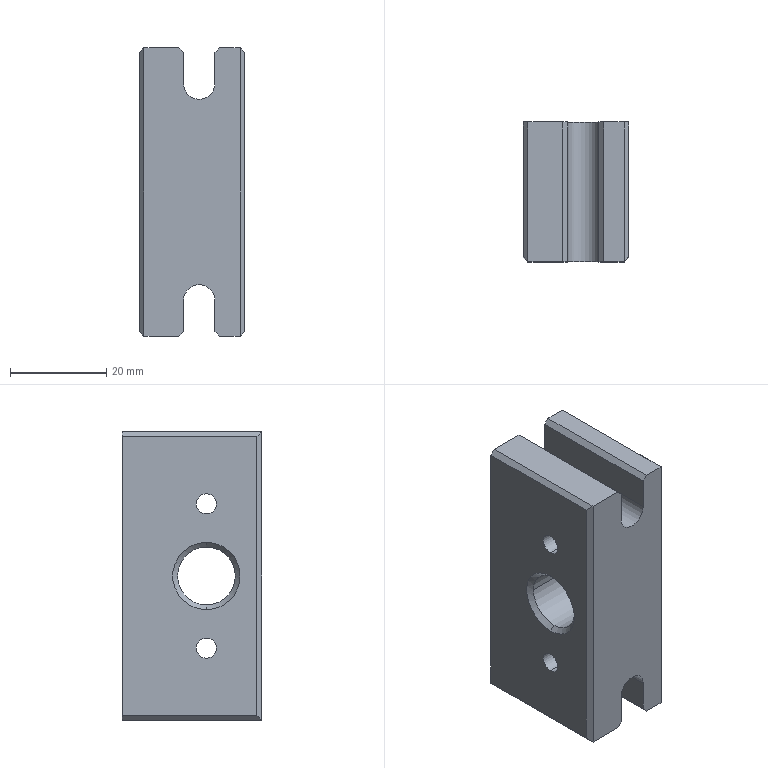Part | STEP file | 602-03-0012 | 1 solid | 35 faces | box 22 x 29 x 60 mm | volume 31178 mm3 | plane 22 | cylinder 9 | cone 4 | commonest cylinder face diameters 4.2 x4 6.5 x3 12 x2